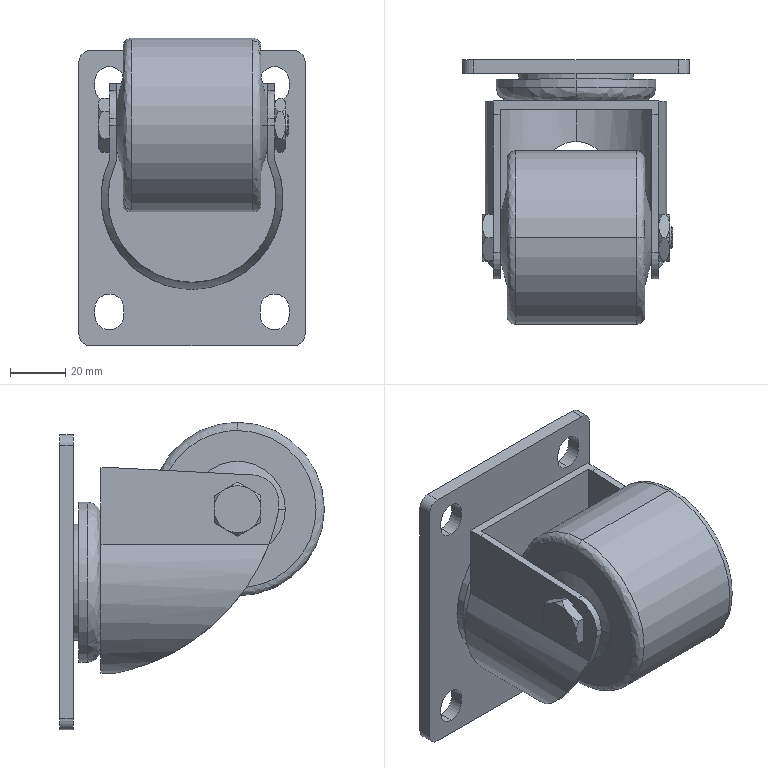Part | SolidWorks | features BaseBody 3 | 3 solids | 119 faces | box 82 x 96 x 111.5 mm | volume 252248 mm3 | plane 49 | cylinder 37 | cone 27 | spline 6 | commonest cylinder face diameters 10.5 x12 8 x6 20 x2 25 x2 40 x2 42 x2